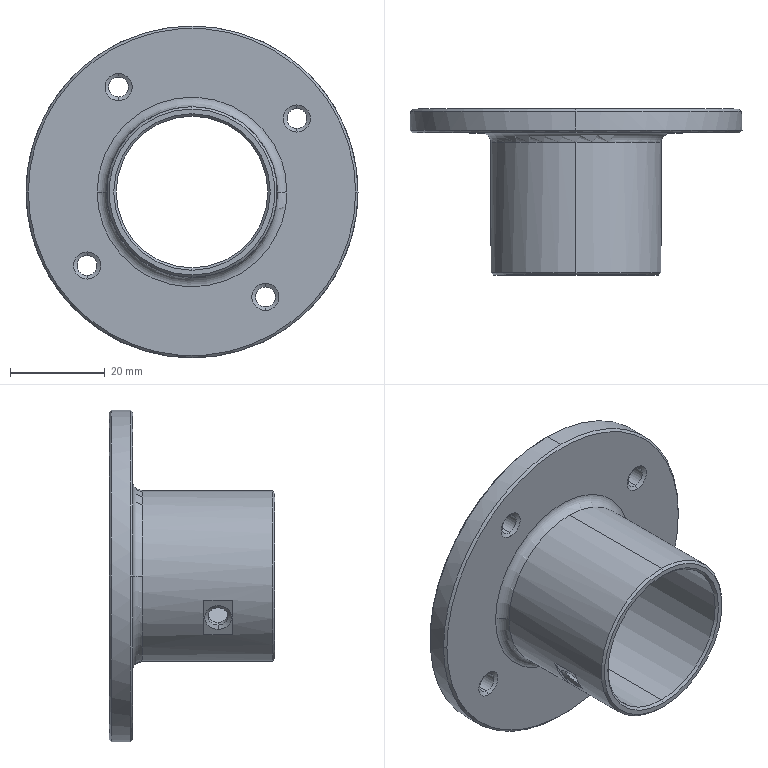Part | STEP file | Support base | 1 solid | 44 faces | box 70 x 35 x 70 mm | volume 21236 mm3 | cone 18 | cylinder 16 | plane 6 | torus 4 | commonest cylinder face diameters 4.2 x10 32 x2 36 x2 70 x2